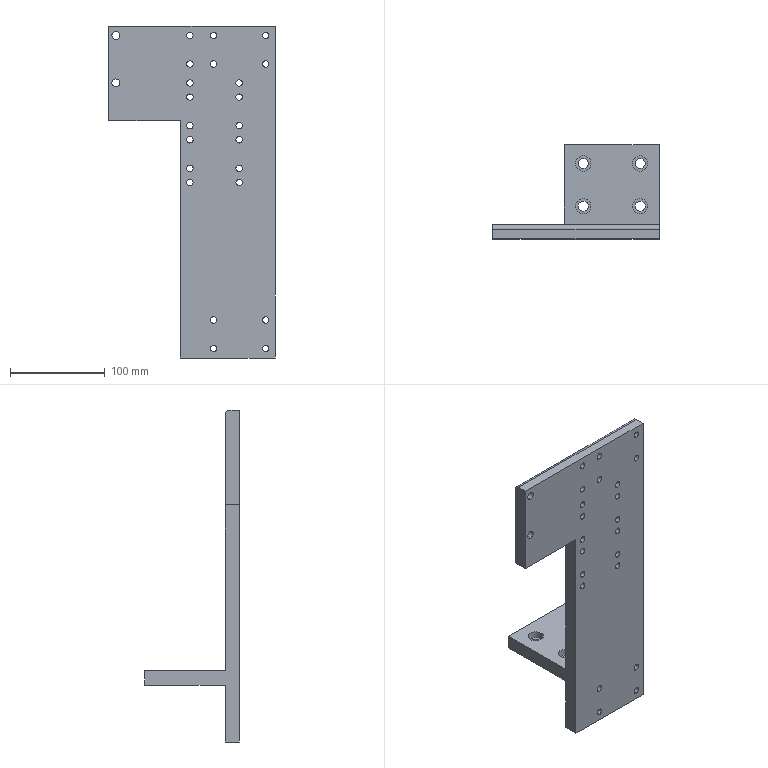Part | SolidWorks | features BaseBody 1 | 1 solid | 81 faces | box 175.5 x 100 x 350 mm | volume 742492 mm3 | cylinder 65 | plane 16 | commonest cylinder face diameters 6.8 x44 10.5 x8 16 x8 8.5 x4 10 x1